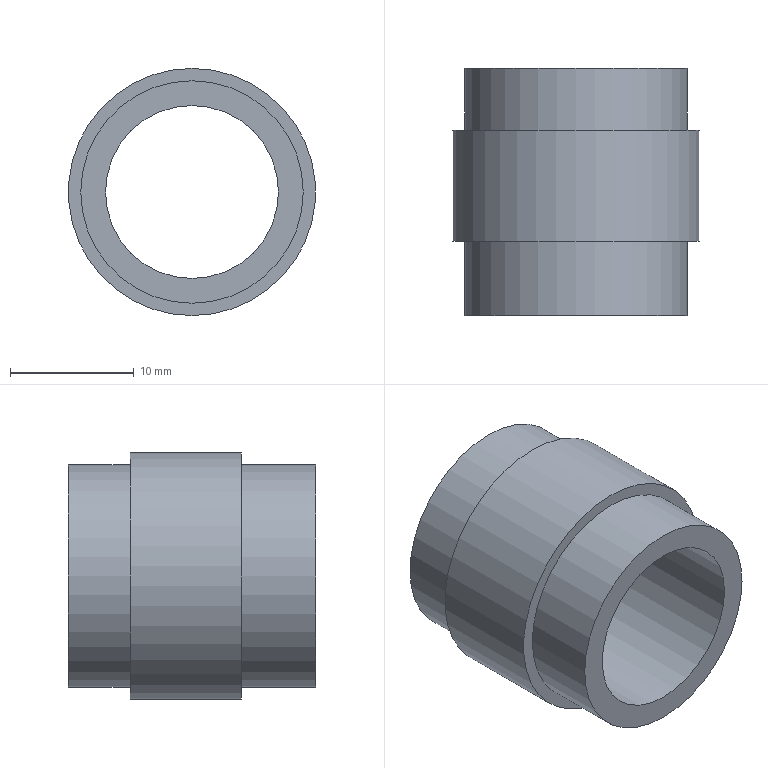Part | STEP file | JBJ-P-1008-04 | 1 solid | 8 faces | box 20 x 20 x 20 mm | volume 2548 mm3 | cylinder 4 | plane 4 | commonest cylinder face diameters 18 x2 14 x1 20 x1
STEP:
#1=CARTESIAN_POINT('',(0.,15.,10.));
#2=VERTEX_POINT('',#1);
#3=CARTESIAN_POINT('',(0.,15.,0.));
#4=DIRECTION('',(0.,1.,0.));
#5=DIRECTION('',(0.,0.,1.));
#6=AXIS2_PLACEMENT_3D('',#3,#4,#5);
#7=CIRCLE('',#6,10.);
#8=EDGE_CURVE('',#2,#2,#7,.T.);
#9=ORIENTED_EDGE('',*,*,#8,.F.);
#10=EDGE_LOOP('',(#9));
#11=FACE_OUTER_BOUND('',#10,.T.);
#12=CARTESIAN_POINT('',(0.,6.,-10.));
#13=VERTEX_POINT('',#12);
#14=CARTESIAN_POINT('',(0.,6.,0.));
#15=DIRECTION('',(0.,-1.,0.));
#16=DIRECTION('',(0.,0.,-1.));
#17=AXIS2_PLACEMENT_3D('',#14,#15,#16);
#18=CIRCLE('',#17,10.);
#19=EDGE_CURVE('',#13,#13,#18,.T.);
#20=ORIENTED_EDGE('',*,*,#19,.F.);
#21=EDGE_LOOP('',(#20));
#22=FACE_OUTER_BOUND('',#21,.T.);
#23=CARTESIAN_POINT('',(0.,20.,0.));
#24=DIRECTION('',(0.,-1.,0.));
#25=DIRECTION('',(0.,0.,-1.));
#26=AXIS2_PLACEMENT_3D('',#23,#24,#25);
#27=CYLINDRICAL_SURFACE('',#26,10.);
#28=ADVANCED_FACE('',(#11,#22),#27,.T.);
#29=CARTESIAN_POINT('',(0.,0.,7.));
#30=VERTEX_POINT('',#29);
#31=CARTESIAN_POINT('',(0.,0.,0.));
#32=DIRECTION('',(0.,1.,0.));
#33=DIRECTION('',(0.,0.,1.));
#34=AXIS2_PLACEMENT_3D('',#31,#32,#33);
#35=CIRCLE('',#34,7.);
#36=EDGE_CURVE('',#30,#30,#35,.T.);
#37=ORIENTED_EDGE('',*,*,#36,.T.);
#38=EDGE_LOOP('',(#37));
#39=FACE_BOUND('',#38,.T.);
#40=CARTESIAN_POINT('',(0.,0.,-9.));
#41=VERTEX_POINT('',#40);
#42=CARTESIAN_POINT('',(0.,0.,0.));
#43=DIRECTION('',(0.,-1.,0.));
#44=DIRECTION('',(0.,0.,-1.));
#45=AXIS2_PLACEMENT_3D('',#42,#43,#44);
#46=CIRCLE('',#45,9.);
#47=EDGE_CURVE('',#41,#41,#46,.T.);
#48=ORIENTED_EDGE('',*,*,#47,.T.);
#49=EDGE_LOOP('',(#48));
#50=FACE_OUTER_BOUND('',#49,.T.);
#51=CARTESIAN_POINT('',(0.,0.,0.));
#52=DIRECTION('',(0.,1.,0.));
#53=DIRECTION('',(0.,0.,1.));
#54=AXIS2_PLACEMENT_3D('',#51,#52,#53);
#55=PLANE('',#54);
#56=ADVANCED_FACE('',(#39,#50),#55,.F.);
#57=CARTESIAN_POINT('',(0.,20.,7.));
#58=VERTEX_POINT('',#57);
#59=CARTESIAN_POINT('',(0.,20.,0.));
#60=DIRECTION('',(0.,1.,0.));
#61=DIRECTION('',(0.,0.,1.));
#62=AXIS2_PLACEMENT_3D('',#59,#60,#61);
#63=CIRCLE('',#62,7.);
#64=EDGE_CURVE('',#58,#58,#63,.T.);
#65=ORIENTED_EDGE('',*,*,#64,.F.);
#66=EDGE_LOOP('',(#65));
#67=FACE_BOUND('',#66,.T.);
#68=CARTESIAN_POINT('',(0.,20.,9.));
#69=VERTEX_POINT('',#68);
#70=CARTESIAN_POINT('',(0.,20.,0.));
#71=DIRECTION('',(0.,1.,0.));
#72=DIRECTION('',(0.,0.,1.));
#73=AXIS2_PLACEMENT_3D('',#70,#71,#72);
#74=CIRCLE('',#73,9.);
#75=EDGE_CURVE('',#69,#69,#74,.T.);
#76=ORIENTED_EDGE('',*,*,#75,.T.);
#77=EDGE_LOOP('',(#76));
#78=FACE_OUTER_BOUND('',#77,.T.);
#79=CARTESIAN_POINT('',(0.,20.,0.));
#80=DIRECTION('',(0.,1.,0.));
#81=DIRECTION('',(0.,0.,1.));
#82=AXIS2_PLACEMENT_3D('',#79,#80,#81);
#83=PLANE('',#82);
#84=ADVANCED_FACE('',(#67,#78),#83,.T.);
#85=ORIENTED_EDGE('',*,*,#64,.T.);
#86=EDGE_LOOP('',(#85));
#87=FACE_OUTER_BOUND('',#86,.T.);
#88=ORIENTED_EDGE('',*,*,#36,.F.);
#89=EDGE_LOOP('',(#88));
#90=FACE_OUTER_BOUND('',#89,.T.);
#91=CARTESIAN_POINT('',(0.,20.,0.));
#92=DIRECTION('',(0.,-1.,0.));
#93=DIRECTION('',(0.,0.,-1.));
#94=AXIS2_PLACEMENT_3D('',#91,#92,#93);
#95=CYLINDRICAL_SURFACE('',#94,7.);
#96=ADVANCED_FACE('',(#87,#90),#95,.F.);
#97=CARTESIAN_POINT('',(0.,15.,9.));
#98=VERTEX_POINT('',#97);
#99=CARTESIAN_POINT('',(0.,15.,0.));
#100=DIRECTION('',(0.,1.,0.));
#101=DIRECTION('',(0.,0.,1.));
#102=AXIS2_PLACEMENT_3D('',#99,#100,#101);
#103=CIRCLE('',#102,9.);
#104=EDGE_CURVE('',#98,#98,#103,.T.);
#105=ORIENTED_EDGE('',*,*,#104,.F.);
#106=EDGE_LOOP('',(#105));
#107=FACE_BOUND('',#106,.T.);
#108=ORIENTED_EDGE('',*,*,#8,.T.);
#109=EDGE_LOOP('',(#108));
#110=FACE_OUTER_BOUND('',#109,.T.);
#111=CARTESIAN_POINT('',(0.,15.,0.));
#112=DIRECTION('',(0.,1.,0.));
#113=DIRECTION('',(0.,0.,1.));
#114=AXIS2_PLACEMENT_3D('',#111,#112,#113);
#115=PLANE('',#114);
#116=ADVANCED_FACE('',(#107,#110),#115,.T.);
#117=ORIENTED_EDGE('',*,*,#104,.T.);
#118=EDGE_LOOP('',(#117));
#119=FACE_OUTER_BOUND('',#118,.T.);
#120=ORIENTED_EDGE('',*,*,#75,.F.);
#121=EDGE_LOOP('',(#120));
#122=FACE_OUTER_BOUND('',#121,.T.);
#123=CARTESIAN_POINT('',(0.,15.,0.));
#124=DIRECTION('',(0.,1.,0.));
#125=DIRECTION('',(0.,0.,1.));
#126=AXIS2_PLACEMENT_3D('',#123,#124,#125);
#127=CYLINDRICAL_SURFACE('',#126,9.);
#128=ADVANCED_FACE('',(#119,#122),#127,.T.);
#129=CARTESIAN_POINT('',(0.,6.,-9.));
#130=VERTEX_POINT('',#129);
#131=CARTESIAN_POINT('',(0.,6.,0.));
#132=DIRECTION('',(0.,-1.,0.));
#133=DIRECTION('',(0.,0.,-1.));
#134=AXIS2_PLACEMENT_3D('',#131,#132,#133);
#135=CIRCLE('',#134,9.);
#136=EDGE_CURVE('',#130,#130,#135,.T.);
#137=ORIENTED_EDGE('',*,*,#136,.F.);
#138=EDGE_LOOP('',(#137));
#139=FACE_BOUND('',#138,.T.);
#140=ORIENTED_EDGE('',*,*,#19,.T.);
#141=EDGE_LOOP('',(#140));
#142=FACE_OUTER_BOUND('',#141,.T.);
#143=CARTESIAN_POINT('',(0.,6.,0.));
#144=DIRECTION('',(0.,-1.,0.));
#145=DIRECTION('',(0.,0.,-1.));
#146=AXIS2_PLACEMENT_3D('',#143,#144,#145);
#147=PLANE('',#146);
#148=ADVANCED_FACE('',(#139,#142),#147,.T.);
#149=ORIENTED_EDGE('',*,*,#136,.T.);
#150=EDGE_LOOP('',(#149));
#151=FACE_OUTER_BOUND('',#150,.T.);
#152=ORIENTED_EDGE('',*,*,#47,.F.);
#153=EDGE_LOOP('',(#152));
#154=FACE_OUTER_BOUND('',#153,.T.);
#155=CARTESIAN_POINT('',(0.,6.,0.));
#156=DIRECTION('',(0.,-1.,0.));
#157=DIRECTION('',(0.,0.,-1.));
#158=AXIS2_PLACEMENT_3D('',#155,#156,#157);
#159=CYLINDRICAL_SURFACE('',#158,9.);
#160=ADVANCED_FACE('',(#151,#154),#159,.T.);
#161=CLOSED_SHELL('',(#28,#56,#84,#96,#116,#128,#148,#160));
#162=MANIFOLD_SOLID_BREP('',#161);
#163=CARTESIAN_POINT('',(0.,0.,0.));
#164=DIRECTION('',(0.,0.,1.));
#165=DIRECTION('',(1.,0.,0.));
#166=AXIS2_PLACEMENT_3D('',#163,#164,#165);
#167=(LENGTH_UNIT()NAMED_UNIT(*)SI_UNIT(.MILLI.,.METRE.));
#168=UNCERTAINTY_MEASURE_WITH_UNIT(LENGTH_MEASURE(0.00001),#167,'','');
#169=(NAMED_UNIT(*)PLANE_ANGLE_UNIT()SI_UNIT($,.RADIAN.));
#170=(NAMED_UNIT(*)SI_UNIT($,.STERADIAN.)SOLID_ANGLE_UNIT());
#171=(GEOMETRIC_REPRESENTATION_CONTEXT(3)GLOBAL_UNCERTAINTY_ASSIGNED_CONTEXT((#168))GLOBAL_UNIT_ASSIGNED_CONTEXT((#167,#169,#170))REPRESENTATION_CONTEXT('',''));
#172=ADVANCED_BREP_SHAPE_REPRESENTATION('',(#162,#166),#171);